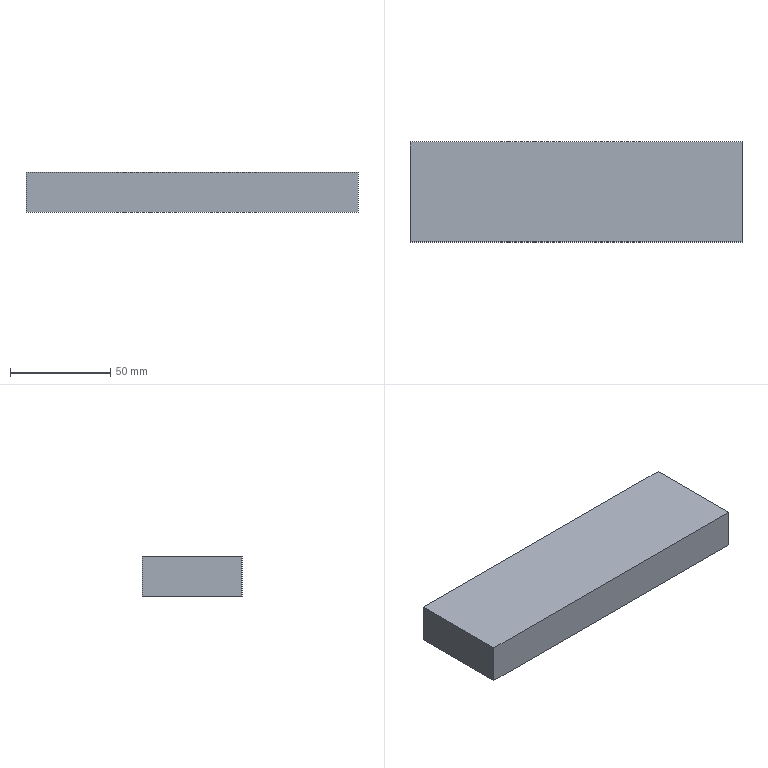Part | SolidWorks | features Extrusion 1 | 1 solid | 6 faces | box 166 x 50 x 20 mm | volume 166000 mm3 | plane 6
STEP:
#1=CARTESIAN_POINT('',(0.,50.,0.));
#2=VERTEX_POINT('',#1);
#3=CARTESIAN_POINT('',(0.,0.,0.));
#4=VERTEX_POINT('',#3);
#5=CARTESIAN_POINT('',(0.,0.,0.));
#6=DIRECTION('',(0.,-1.,0.));
#7=VECTOR('',#6,1000.);
#8=LINE('',#5,#7);
#9=EDGE_CURVE('',#2,#4,#8,.T.);
#10=ORIENTED_EDGE('',*,*,#9,.T.);
#11=CARTESIAN_POINT('',(0.,0.,20.));
#12=VERTEX_POINT('',#11);
#13=CARTESIAN_POINT('',(0.,0.,20.));
#14=DIRECTION('',(0.,0.,-1.));
#15=VECTOR('',#14,1000.);
#16=LINE('',#13,#15);
#17=EDGE_CURVE('',#12,#4,#16,.T.);
#18=ORIENTED_EDGE('',*,*,#17,.F.);
#19=CARTESIAN_POINT('',(0.,50.,20.));
#20=VERTEX_POINT('',#19);
#21=CARTESIAN_POINT('',(0.,0.,20.));
#22=DIRECTION('',(0.,-1.,0.));
#23=VECTOR('',#22,1000.);
#24=LINE('',#21,#23);
#25=EDGE_CURVE('',#20,#12,#24,.T.);
#26=ORIENTED_EDGE('',*,*,#25,.F.);
#27=CARTESIAN_POINT('',(0.,50.,20.));
#28=DIRECTION('',(0.,0.,-1.));
#29=VECTOR('',#28,1000.);
#30=LINE('',#27,#29);
#31=EDGE_CURVE('',#20,#2,#30,.T.);
#32=ORIENTED_EDGE('',*,*,#31,.T.);
#33=EDGE_LOOP('',(#10,#18,#26,#32));
#34=FACE_OUTER_BOUND('',#33,.T.);
#35=CARTESIAN_POINT('',(0.,0.,20.));
#36=DIRECTION('',(1.,0.,0.));
#37=DIRECTION('',(0.,0.,-1.));
#38=AXIS2_PLACEMENT_3D('',#35,#36,#37);
#39=PLANE('',#38);
#40=ADVANCED_FACE('',(#34),#39,.F.);
#41=CARTESIAN_POINT('',(166.,0.,0.));
#42=VERTEX_POINT('',#41);
#43=CARTESIAN_POINT('',(0.,0.,0.));
#44=DIRECTION('',(1.,0.,0.));
#45=VECTOR('',#44,1000.);
#46=LINE('',#43,#45);
#47=EDGE_CURVE('',#4,#42,#46,.T.);
#48=ORIENTED_EDGE('',*,*,#47,.T.);
#49=CARTESIAN_POINT('',(166.,0.,20.));
#50=VERTEX_POINT('',#49);
#51=CARTESIAN_POINT('',(166.,0.,20.));
#52=DIRECTION('',(0.,0.,-1.));
#53=VECTOR('',#52,1000.);
#54=LINE('',#51,#53);
#55=EDGE_CURVE('',#50,#42,#54,.T.);
#56=ORIENTED_EDGE('',*,*,#55,.F.);
#57=CARTESIAN_POINT('',(0.,0.,20.));
#58=DIRECTION('',(1.,0.,0.));
#59=VECTOR('',#58,1000.);
#60=LINE('',#57,#59);
#61=EDGE_CURVE('',#12,#50,#60,.T.);
#62=ORIENTED_EDGE('',*,*,#61,.F.);
#63=ORIENTED_EDGE('',*,*,#17,.T.);
#64=EDGE_LOOP('',(#48,#56,#62,#63));
#65=FACE_OUTER_BOUND('',#64,.T.);
#66=CARTESIAN_POINT('',(0.,0.,20.));
#67=DIRECTION('',(0.,1.,0.));
#68=DIRECTION('',(0.,0.,1.));
#69=AXIS2_PLACEMENT_3D('',#66,#67,#68);
#70=PLANE('',#69);
#71=ADVANCED_FACE('',(#65),#70,.F.);
#72=CARTESIAN_POINT('',(166.,50.,0.));
#73=VERTEX_POINT('',#72);
#74=CARTESIAN_POINT('',(166.,0.,0.));
#75=DIRECTION('',(0.,1.,0.));
#76=VECTOR('',#75,1000.);
#77=LINE('',#74,#76);
#78=EDGE_CURVE('',#42,#73,#77,.T.);
#79=ORIENTED_EDGE('',*,*,#78,.T.);
#80=CARTESIAN_POINT('',(166.,50.,20.));
#81=VERTEX_POINT('',#80);
#82=CARTESIAN_POINT('',(166.,50.,20.));
#83=DIRECTION('',(0.,0.,-1.));
#84=VECTOR('',#83,1000.);
#85=LINE('',#82,#84);
#86=EDGE_CURVE('',#81,#73,#85,.T.);
#87=ORIENTED_EDGE('',*,*,#86,.F.);
#88=CARTESIAN_POINT('',(166.,0.,20.));
#89=DIRECTION('',(0.,1.,0.));
#90=VECTOR('',#89,1000.);
#91=LINE('',#88,#90);
#92=EDGE_CURVE('',#50,#81,#91,.T.);
#93=ORIENTED_EDGE('',*,*,#92,.F.);
#94=ORIENTED_EDGE('',*,*,#55,.T.);
#95=EDGE_LOOP('',(#79,#87,#93,#94));
#96=FACE_OUTER_BOUND('',#95,.T.);
#97=CARTESIAN_POINT('',(166.,0.,20.));
#98=DIRECTION('',(-1.,0.,0.));
#99=DIRECTION('',(0.,0.,1.));
#100=AXIS2_PLACEMENT_3D('',#97,#98,#99);
#101=PLANE('',#100);
#102=ADVANCED_FACE('',(#96),#101,.F.);
#103=CARTESIAN_POINT('',(0.,50.,0.));
#104=DIRECTION('',(-1.,0.,0.));
#105=VECTOR('',#104,1000.);
#106=LINE('',#103,#105);
#107=EDGE_CURVE('',#73,#2,#106,.T.);
#108=ORIENTED_EDGE('',*,*,#107,.T.);
#109=ORIENTED_EDGE('',*,*,#31,.F.);
#110=CARTESIAN_POINT('',(0.,50.,20.));
#111=DIRECTION('',(-1.,0.,0.));
#112=VECTOR('',#111,1000.);
#113=LINE('',#110,#112);
#114=EDGE_CURVE('',#81,#20,#113,.T.);
#115=ORIENTED_EDGE('',*,*,#114,.F.);
#116=ORIENTED_EDGE('',*,*,#86,.T.);
#117=EDGE_LOOP('',(#108,#109,#115,#116));
#118=FACE_OUTER_BOUND('',#117,.T.);
#119=CARTESIAN_POINT('',(0.,50.,20.));
#120=DIRECTION('',(0.,-1.,0.));
#121=DIRECTION('',(0.,0.,-1.));
#122=AXIS2_PLACEMENT_3D('',#119,#120,#121);
#123=PLANE('',#122);
#124=ADVANCED_FACE('',(#118),#123,.F.);
#125=ORIENTED_EDGE('',*,*,#25,.T.);
#126=ORIENTED_EDGE('',*,*,#61,.T.);
#127=ORIENTED_EDGE('',*,*,#92,.T.);
#128=ORIENTED_EDGE('',*,*,#114,.T.);
#129=EDGE_LOOP('',(#125,#126,#127,#128));
#130=FACE_OUTER_BOUND('',#129,.T.);
#131=CARTESIAN_POINT('',(0.,0.,20.));
#132=DIRECTION('',(0.,0.,-1.));
#133=DIRECTION('',(-1.,0.,0.));
#134=AXIS2_PLACEMENT_3D('',#131,#132,#133);
#135=PLANE('',#134);
#136=ADVANCED_FACE('',(#130),#135,.F.);
#137=ORIENTED_EDGE('',*,*,#9,.F.);
#138=ORIENTED_EDGE('',*,*,#107,.F.);
#139=ORIENTED_EDGE('',*,*,#78,.F.);
#140=ORIENTED_EDGE('',*,*,#47,.F.);
#141=EDGE_LOOP('',(#137,#138,#139,#140));
#142=FACE_OUTER_BOUND('',#141,.T.);
#143=CARTESIAN_POINT('',(0.,0.,0.));
#144=DIRECTION('',(0.,0.,-1.));
#145=DIRECTION('',(-1.,0.,0.));
#146=AXIS2_PLACEMENT_3D('',#143,#144,#145);
#147=PLANE('',#146);
#148=ADVANCED_FACE('',(#142),#147,.T.);
#149=CLOSED_SHELL('',(#40,#71,#102,#124,#136,#148));
#150=MANIFOLD_SOLID_BREP('',#149);
#151=CARTESIAN_POINT('',(0.,0.,0.));
#152=DIRECTION('',(0.,0.,1.));
#153=DIRECTION('',(1.,0.,0.));
#154=AXIS2_PLACEMENT_3D('',#151,#152,#153);
#155=(LENGTH_UNIT()NAMED_UNIT(*)SI_UNIT(.MILLI.,.METRE.));
#156=UNCERTAINTY_MEASURE_WITH_UNIT(LENGTH_MEASURE(0.00001),#155,'','');
#157=(NAMED_UNIT(*)PLANE_ANGLE_UNIT()SI_UNIT($,.RADIAN.));
#158=(NAMED_UNIT(*)SI_UNIT($,.STERADIAN.)SOLID_ANGLE_UNIT());
#159=(GEOMETRIC_REPRESENTATION_CONTEXT(3)GLOBAL_UNCERTAINTY_ASSIGNED_CONTEXT((#156))GLOBAL_UNIT_ASSIGNED_CONTEXT((#155,#157,#158))REPRESENTATION_CONTEXT('',''));
#160=ADVANCED_BREP_SHAPE_REPRESENTATION('',(#150,#154),#159);